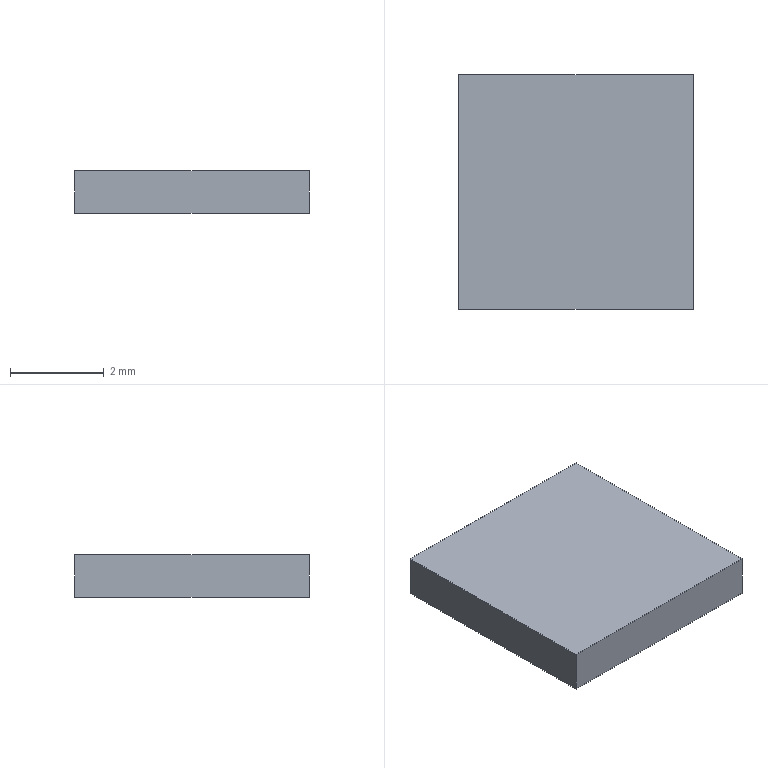Part | Creo | 1 solid | 6 faces | box 5 x 5 x 0.8999 mm | volume 22.498 mm3 | plane 6
STEP:
#1=CARTESIAN_POINT('',(0.,0.,0.));
#2=DIRECTION('',(0.,0.,1.));
#3=DIRECTION('',(1.,0.,0.));
#4=AXIS2_PLACEMENT_3D('',#1,#2,#3);
#5=CARTESIAN_POINT('',(-2.5,2.5,0.));
#6=VERTEX_POINT('',#5);
#7=CARTESIAN_POINT('',(-2.5,-2.5,0.));
#8=VERTEX_POINT('',#7);
#9=CARTESIAN_POINT('',(-2.5,2.5,0.));
#10=DIRECTION('',(0.,-1.,0.));
#11=VECTOR('',#10,5.);
#12=LINE('',#9,#11);
#13=EDGE_CURVE('',#6,#8,#12,.T.);
#14=ORIENTED_EDGE('',*,*,#13,.T.);
#15=CARTESIAN_POINT('',(2.5,-2.5,0.));
#16=VERTEX_POINT('',#15);
#17=CARTESIAN_POINT('',(-2.5,-2.5,0.));
#18=DIRECTION('',(1.,0.,0.));
#19=VECTOR('',#18,5.);
#20=LINE('',#17,#19);
#21=EDGE_CURVE('',#8,#16,#20,.T.);
#22=ORIENTED_EDGE('',*,*,#21,.T.);
#23=CARTESIAN_POINT('',(2.5,2.5,0.));
#24=VERTEX_POINT('',#23);
#25=CARTESIAN_POINT('',(2.5,-2.5,0.));
#26=DIRECTION('',(0.,1.,0.));
#27=VECTOR('',#26,5.);
#28=LINE('',#25,#27);
#29=EDGE_CURVE('',#16,#24,#28,.T.);
#30=ORIENTED_EDGE('',*,*,#29,.T.);
#31=CARTESIAN_POINT('',(2.5,2.5,0.));
#32=DIRECTION('',(-1.,0.,0.));
#33=VECTOR('',#32,5.);
#34=LINE('',#31,#33);
#35=EDGE_CURVE('',#24,#6,#34,.T.);
#36=ORIENTED_EDGE('',*,*,#35,.T.);
#37=EDGE_LOOP('',(#14,#22,#30,#36));
#38=FACE_OUTER_BOUND('',#37,.F.);
#39=CARTESIAN_POINT('',(0.,0.,0.));
#40=DIRECTION('',(0.,0.,1.));
#41=DIRECTION('',(1.,0.,0.));
#42=AXIS2_PLACEMENT_3D('',#39,#40,#41);
#43=PLANE('',#42);
#44=ADVANCED_FACE('',(#38),#43,.F.);
#45=ORIENTED_EDGE('',*,*,#13,.F.);
#46=CARTESIAN_POINT('',(-2.5,2.5,0.8999));
#47=VERTEX_POINT('',#46);
#48=CARTESIAN_POINT('',(-2.5,2.5,0.));
#49=DIRECTION('',(0.,0.,1.));
#50=VECTOR('',#49,0.8999);
#51=LINE('',#48,#50);
#52=EDGE_CURVE('',#6,#47,#51,.T.);
#53=ORIENTED_EDGE('',*,*,#52,.T.);
#54=CARTESIAN_POINT('',(-2.5,-2.5,0.8999));
#55=VERTEX_POINT('',#54);
#56=CARTESIAN_POINT('',(-2.5,2.5,0.8999));
#57=DIRECTION('',(0.,-1.,0.));
#58=VECTOR('',#57,5.);
#59=LINE('',#56,#58);
#60=EDGE_CURVE('',#47,#55,#59,.T.);
#61=ORIENTED_EDGE('',*,*,#60,.T.);
#62=CARTESIAN_POINT('',(-2.5,-2.5,0.));
#63=DIRECTION('',(0.,0.,1.));
#64=VECTOR('',#63,0.8999);
#65=LINE('',#62,#64);
#66=EDGE_CURVE('',#8,#55,#65,.T.);
#67=ORIENTED_EDGE('',*,*,#66,.F.);
#68=EDGE_LOOP('',(#45,#53,#61,#67));
#69=FACE_OUTER_BOUND('',#68,.F.);
#70=CARTESIAN_POINT('',(-2.5,2.5,0.));
#71=DIRECTION('',(-1.,0.,0.));
#72=DIRECTION('',(0.,-1.,0.));
#73=AXIS2_PLACEMENT_3D('',#70,#71,#72);
#74=PLANE('',#73);
#75=ADVANCED_FACE('',(#69),#74,.T.);
#76=ORIENTED_EDGE('',*,*,#35,.F.);
#77=CARTESIAN_POINT('',(2.5,2.5,0.8999));
#78=VERTEX_POINT('',#77);
#79=CARTESIAN_POINT('',(2.5,2.5,0.));
#80=DIRECTION('',(0.,0.,1.));
#81=VECTOR('',#80,0.8999);
#82=LINE('',#79,#81);
#83=EDGE_CURVE('',#24,#78,#82,.T.);
#84=ORIENTED_EDGE('',*,*,#83,.T.);
#85=CARTESIAN_POINT('',(2.5,2.5,0.8999));
#86=DIRECTION('',(-1.,0.,0.));
#87=VECTOR('',#86,5.);
#88=LINE('',#85,#87);
#89=EDGE_CURVE('',#78,#47,#88,.T.);
#90=ORIENTED_EDGE('',*,*,#89,.T.);
#91=ORIENTED_EDGE('',*,*,#52,.F.);
#92=EDGE_LOOP('',(#76,#84,#90,#91));
#93=FACE_OUTER_BOUND('',#92,.F.);
#94=CARTESIAN_POINT('',(2.5,2.5,0.));
#95=DIRECTION('',(0.,1.,0.));
#96=DIRECTION('',(-1.,0.,0.));
#97=AXIS2_PLACEMENT_3D('',#94,#95,#96);
#98=PLANE('',#97);
#99=ADVANCED_FACE('',(#93),#98,.T.);
#100=ORIENTED_EDGE('',*,*,#29,.F.);
#101=CARTESIAN_POINT('',(2.5,-2.5,0.8999));
#102=VERTEX_POINT('',#101);
#103=CARTESIAN_POINT('',(2.5,-2.5,0.));
#104=DIRECTION('',(0.,0.,1.));
#105=VECTOR('',#104,0.8999);
#106=LINE('',#103,#105);
#107=EDGE_CURVE('',#16,#102,#106,.T.);
#108=ORIENTED_EDGE('',*,*,#107,.T.);
#109=CARTESIAN_POINT('',(2.5,-2.5,0.8999));
#110=DIRECTION('',(0.,1.,0.));
#111=VECTOR('',#110,5.);
#112=LINE('',#109,#111);
#113=EDGE_CURVE('',#102,#78,#112,.T.);
#114=ORIENTED_EDGE('',*,*,#113,.T.);
#115=ORIENTED_EDGE('',*,*,#83,.F.);
#116=EDGE_LOOP('',(#100,#108,#114,#115));
#117=FACE_OUTER_BOUND('',#116,.F.);
#118=CARTESIAN_POINT('',(2.5,-2.5,0.));
#119=DIRECTION('',(1.,0.,0.));
#120=DIRECTION('',(0.,1.,0.));
#121=AXIS2_PLACEMENT_3D('',#118,#119,#120);
#122=PLANE('',#121);
#123=ADVANCED_FACE('',(#117),#122,.T.);
#124=ORIENTED_EDGE('',*,*,#21,.F.);
#125=ORIENTED_EDGE('',*,*,#66,.T.);
#126=CARTESIAN_POINT('',(-2.5,-2.5,0.8999));
#127=DIRECTION('',(1.,0.,0.));
#128=VECTOR('',#127,5.);
#129=LINE('',#126,#128);
#130=EDGE_CURVE('',#55,#102,#129,.T.);
#131=ORIENTED_EDGE('',*,*,#130,.T.);
#132=ORIENTED_EDGE('',*,*,#107,.F.);
#133=EDGE_LOOP('',(#124,#125,#131,#132));
#134=FACE_OUTER_BOUND('',#133,.F.);
#135=CARTESIAN_POINT('',(-2.5,-2.5,0.));
#136=DIRECTION('',(0.,-1.,0.));
#137=DIRECTION('',(1.,0.,0.));
#138=AXIS2_PLACEMENT_3D('',#135,#136,#137);
#139=PLANE('',#138);
#140=ADVANCED_FACE('',(#134),#139,.T.);
#141=ORIENTED_EDGE('',*,*,#60,.F.);
#142=ORIENTED_EDGE('',*,*,#89,.F.);
#143=ORIENTED_EDGE('',*,*,#113,.F.);
#144=ORIENTED_EDGE('',*,*,#130,.F.);
#145=EDGE_LOOP('',(#141,#142,#143,#144));
#146=FACE_OUTER_BOUND('',#145,.F.);
#147=CARTESIAN_POINT('',(0.,0.,0.8999));
#148=DIRECTION('',(0.,0.,1.));
#149=DIRECTION('',(1.,0.,0.));
#150=AXIS2_PLACEMENT_3D('',#147,#148,#149);
#151=PLANE('',#150);
#152=ADVANCED_FACE('',(#146),#151,.T.);
#153=CLOSED_SHELL('',(#44,#75,#99,#123,#140,#152));
#154=MANIFOLD_SOLID_BREP('',#153);
#155=(LENGTH_UNIT()NAMED_UNIT(*)SI_UNIT(.MILLI.,.METRE.));
#156=UNCERTAINTY_MEASURE_WITH_UNIT(LENGTH_MEASURE(0.0007128),#155,'','');
#157=(NAMED_UNIT(*)PLANE_ANGLE_UNIT()SI_UNIT($,.RADIAN.));
#158=PLANE_ANGLE_MEASURE_WITH_UNIT(PLANE_ANGLE_MEASURE(0.01745),#157);
#159=(CONVERSION_BASED_UNIT('DEGREE',#158)NAMED_UNIT(*)PLANE_ANGLE_UNIT());
#160=(NAMED_UNIT(*)SI_UNIT($,.STERADIAN.)SOLID_ANGLE_UNIT());
#161=(GEOMETRIC_REPRESENTATION_CONTEXT(3)GLOBAL_UNCERTAINTY_ASSIGNED_CONTEXT((#156))GLOBAL_UNIT_ASSIGNED_CONTEXT((#155,#159,#160))REPRESENTATION_CONTEXT('',''));
#162=ADVANCED_BREP_SHAPE_REPRESENTATION('',(#4,#154),#161);